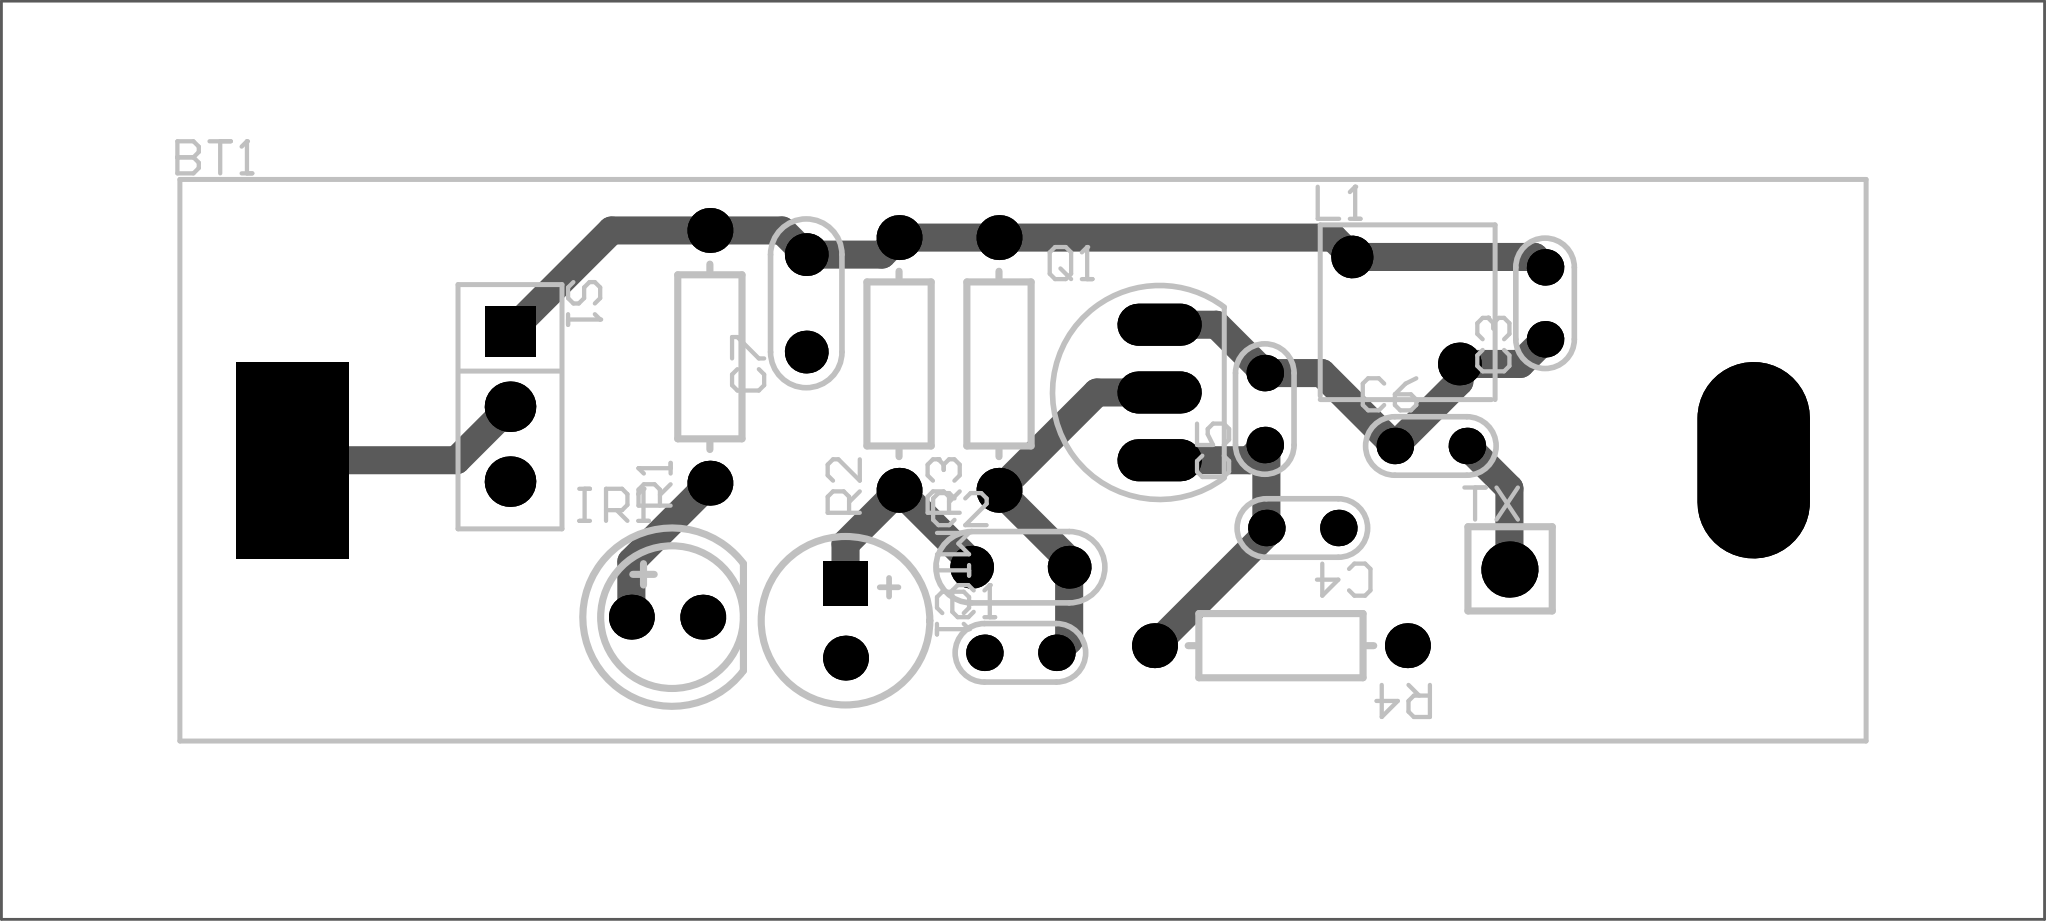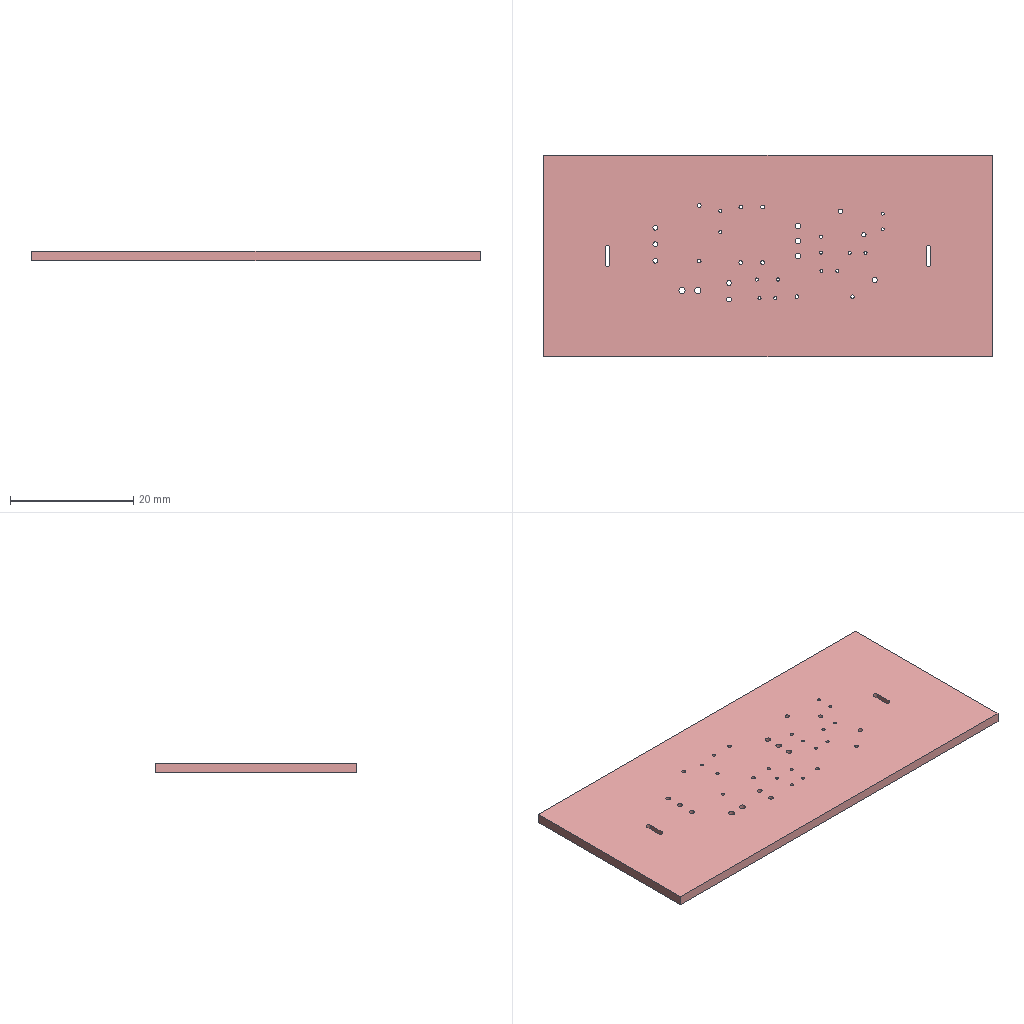Circuit board layout | Altium Designer | box 72.7 x 32.7 x 1.6 mm
Layer stack:
# Altium Designer layer stack of  (unit mm; dielectric type: 0 none, 1 core, 2 prepreg, 3 surface material)
index,name,kind,layer,copper_thickness_mm,dielectric_type,dielectric_thickness_mm,dielectric_material,dielectric_constant
0,Top Paste Mask Layer,other,,,,,,
1,Top Silkscreen Layer,other,,,,,,
2,Top Solder Mask Layer,dielectric,,,3,0.01,,3.3
3,Top Layer,copper,Top Layer,0.035,,,,
4,Dielectric1,dielectric,,,3,1.51,FR4,4.5
5,Bottom Layer,copper,Bottom Layer,0.035,,,,
6,Bottom Solder Mask Layer,dielectric,,,3,0.01,,3.3
7,Bottom Silkscreen Layer,other,,,,,,
8,Bottom Paste Mask Layer,other,,,,,,
# drill layer pairs: low layer,high layer
drill_pair,Top Layer,Bottom Layer
Part placement:
Designator,Comment,Layer,Footprint,Center-X(mm),Center-Y(mm),Rotation
BT1,BATTERY,TopLayer,Bat_Box_01,106.2,86.2,0
C1,103,TopLayer,CC_1.8*3.6,106.108,79.342,0
C2,104,TopLayer,CC_2.2*5,106.108,82.39,0
C3,30pf,TopLayer,CC_1.8*3.6,124.777,91.788,90
C4,30pf,TopLayer,CC_1.8*3.6,116.141,83.787,180
C5,10pf,TopLayer,CC_1.8*3.6,114.803,88.023,90
C6,30pf,TopLayer,CC_1.8*3.6,120.713,86.708,0
C7,104,TopLayer,CC_2.2*5,98.488,91.788,90
IR1,LED_R_L,TopLayer,LED-TH_BD5.0-P2.54-FD,93.535,80.612,0
L1,4T,TopLayer,IND_5x5,119.824,91.534,0
MIC1,MIC,TopLayer,MIC-TH_BD6.0-P1.90-D0.4-L-FD_GMI6050P-2CXXDB,99.885,80.485,270
Q1,9018,TopLayer,TANS,111.061,88.613,0
R1,Res,TopLayer,AXIAL0.4-1/4W,95.059,89.883,90
R2,Res,TopLayer,AXIAL0.4-1/4W,101.79,89.629,90
R3,Res,TopLayer,AXIAL0.4-1/4W,105.346,89.629,90
R4,Res,TopLayer,AXIAL0.4-1/4W,115.379,79.596,180
S1,MTS-10x,TopLayer,SW-TH_KH-SS12D01-G3-5.0,87.947,88.105,270
TX,TX,TopLayer,TX,123.509,82.308,0
Pad and via stacks:
# Altium Designer via and pad stacks of  (unit mm). Each distinct definition once, with the count of objects using it.
# via: kind,start_layer,end_layer,hole_mm,diameter_mm,mode(0 simple;1 top-mid-bottom;2 full stack),diameter_per_layer,count,example_net
# pad: kind,layer,hole_mm,hole_type(0 round;1 square;2 slot),plating,top_size,top_shape(1 round;2 rect;3 octagon;9 rounded rect),mid_size,bottom_size,mode,footprint,size_per_layer,count,example
pad,Multi-Layer,0.8,2,plated,7x4,1,7x4,7x4,0,Bat_Box_01,,1,BT1.2
pad,Multi-Layer,0.8,2,plated,7x4,2,7x4,7x4,0,Bat_Box_01,,1,BT1.1
pad,Multi-Layer,0.5,0,plated,1.3x1.3,1,1.3x1.3,1.3x1.3,0,CC 1.8*3.6,,10,C1.2
pad,Multi-Layer,0.5,0,plated,1.524x1.524,1,1.524x1.524,1.524x1.524,0,CC 2.2*5,,4,C2.1
pad,Multi-Layer,1,0,plated,1.6x1.6,1,1.6x1.6,1.6x1.6,0,LED-TH_BD5.0-P2.54-FD,,2,IR1.1
pad,Multi-Layer,0.7112,0,plated,1.524x1.524,1,1.524x1.524,1.524x1.524,0,IND_5x5,,1,L1.2
pad,Multi-Layer,0.7112,0,plated,1.524x1.5,1,1.524x1.5,1.524x1.5,0,IND_5x5,,1,L1.1
pad,Multi-Layer,0.8,0,plated,1.6x1.6,1,1.6x1.6,1.6x1.6,0,MIC-TH_BD6.0-P1.90-D0.4-L-FD_GMI6050P-2CXXDB,,1,MIC1.2
pad,Multi-Layer,0.8,0,plated,1.6x1.6,2,1.6x1.6,1.6x1.6,0,MIC-TH_BD6.0-P1.90-D0.4-L-FD_GMI6050P-2CXXDB,,1,MIC1.1
pad,Multi-Layer,0.9,0,plated,3x1.5,1,3x1.5,3x1.5,0,TANS,,3,Q1.1
pad,Multi-Layer,0.6,0,plated,1.6x1.6,1,1.6x1.6,1.6x1.6,0,AXIAL0.4-1/4W,,8,R1.2
pad,Multi-Layer,0.8,0,plated,1.8x1.8,2,1.8x1.8,1.8x1.8,0,SW-TH_KH-SS12D01-G3-5.0,,1,S1.1
pad,Multi-Layer,0.8,0,plated,1.8x1.8,1,1.8x1.8,1.8x1.8,0,SW-TH_KH-SS12D01-G3-5.0,,2,S1.2
pad,Multi-Layer,0.8,0,plated,2x2,1,2x2,2x2,0,TX,,1,TX.1
Design rules, without the lines most boards share:
# Altium Designer design rules of  (exported by Altium Designer, unit mm)
# columns: name | kind | enabled | priority | scope1 | scope2 | descriptor | typed fields (field=value)
copperThickness1oz_2 | 2 | enabled | 2 | All | All | Width Constraint (Min=5mil) (Max=100mil) (Preferred=39.4mil) (All) |